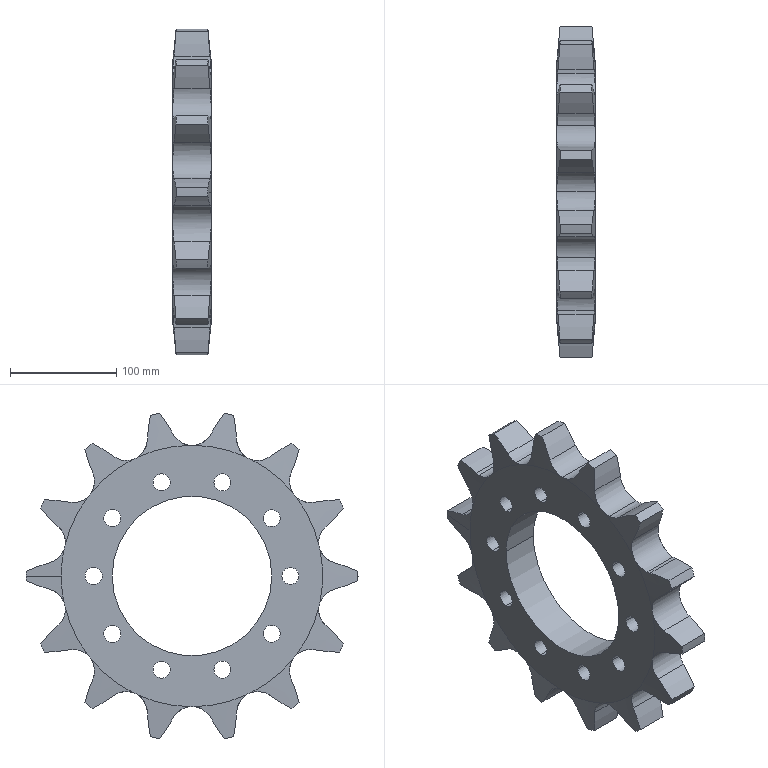Part | SolidWorks | features ICE 2, CirPattern 1, Revolution 1 | 1 solid | 116 faces | box 36 x 312 x 306.035 mm | volume 1353964 mm3 | cylinder 84 | cone 30 | plane 2 | commonest cylinder face diameters 288.24 x28 16 x20 39.98 x19 312 x15 150 x2